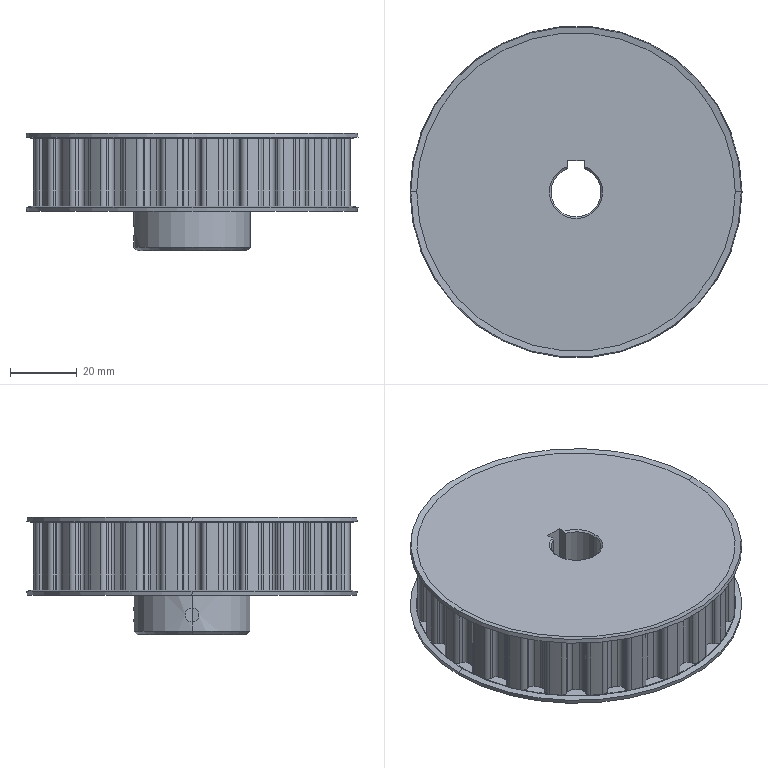Part | STEP file | Timing pulley 2_3 | 1 solid | 297 faces | box 99.713 x 99.713 x 35.319 mm | volume 162767 mm3 | cylinder 147 | plane 126 | cone 20 | spline 4 | commonest cylinder face diameters 3.2 x114 95.649 x24 4.134 x4 15 x3 35 x2